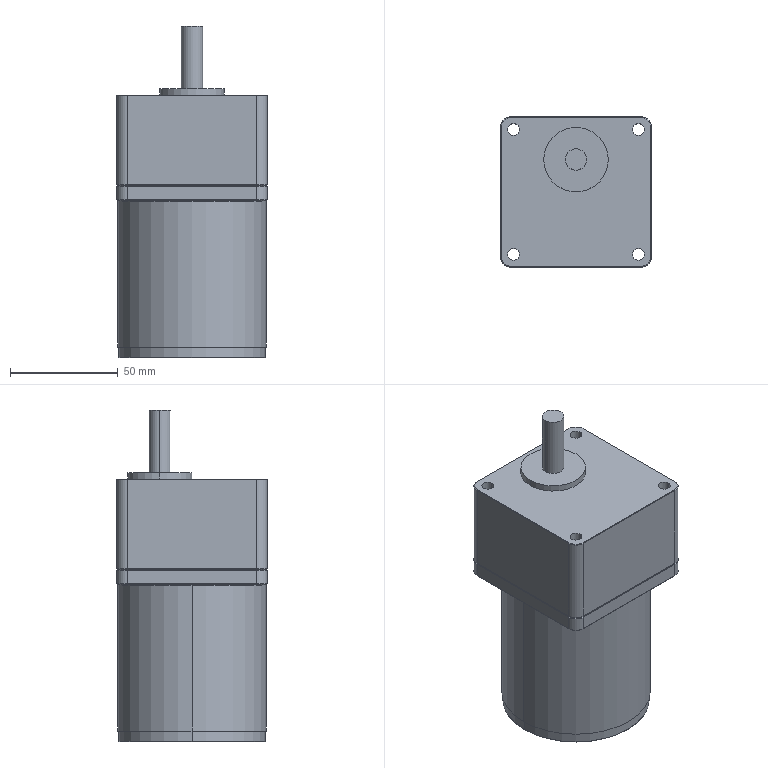Part | NX | 1 solid | 102 faces | box 70 x 70 x 154 mm | volume 511145 mm3 | cone 36 | plane 34 | cylinder 32 | commonest cylinder face diameters 5.5 x16 10 x10 30 x2 68 x2 69 x2